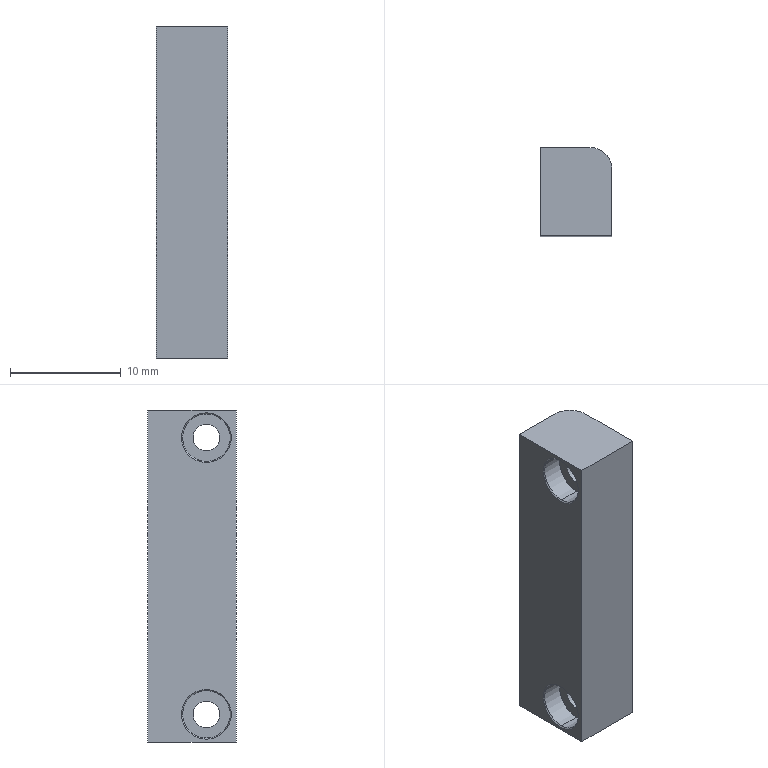Part | SolidWorks | features HoleWzd 2, Chamfer 1, Extrusion 1, Fillet 1 | 1 solid | 27 faces | box 6.5 x 8 x 30 mm | volume 1393 mm3 | cylinder 13 | plane 10 | cone 4 | commonest cylinder face diameters 2.4 x4 3 x4 4.3 x4 4 x1
STEP:
#1=CARTESIAN_POINT('',(-3.153,-1.3,0.35));
#2=VERTEX_POINT('',#1);
#3=CARTESIAN_POINT('',(-3.153,-1.3,4.65));
#4=VERTEX_POINT('',#3);
#5=CARTESIAN_POINT('',(-3.153,-1.3,2.5));
#6=DIRECTION('',(-1.,0.,0.));
#7=DIRECTION('',(0.,0.,-1.));
#8=AXIS2_PLACEMENT_3D('',#5,#6,#7);
#9=CIRCLE('',#8,2.15);
#10=EDGE_CURVE('',#2,#4,#9,.T.);
#11=ORIENTED_EDGE('',*,*,#10,.F.);
#12=CARTESIAN_POINT('',(-3.25,-1.3,0.25));
#13=VERTEX_POINT('',#12);
#14=CARTESIAN_POINT('',(-3.153,-1.3,0.35));
#15=DIRECTION('',(-0.6947,0.,-0.7193));
#16=VECTOR('',#15,1000.);
#17=LINE('',#14,#16);
#18=EDGE_CURVE('',#2,#13,#17,.T.);
#19=ORIENTED_EDGE('',*,*,#18,.T.);
#20=CARTESIAN_POINT('',(-3.25,-1.3,4.75));
#21=VERTEX_POINT('',#20);
#22=CARTESIAN_POINT('',(-3.25,-1.3,2.5));
#23=DIRECTION('',(1.,0.,0.));
#24=DIRECTION('',(0.,0.,-1.));
#25=AXIS2_PLACEMENT_3D('',#22,#23,#24);
#26=CIRCLE('',#25,2.25);
#27=EDGE_CURVE('',#21,#13,#26,.T.);
#28=ORIENTED_EDGE('',*,*,#27,.F.);
#29=CARTESIAN_POINT('',(-3.153,-1.3,4.65));
#30=DIRECTION('',(-0.6947,0.,0.7193));
#31=VECTOR('',#30,1000.);
#32=LINE('',#29,#31);
#33=EDGE_CURVE('',#4,#21,#32,.T.);
#34=ORIENTED_EDGE('',*,*,#33,.F.);
#35=EDGE_LOOP('',(#11,#19,#28,#34));
#36=FACE_OUTER_BOUND('',#35,.T.);
#37=CARTESIAN_POINT('',(-3.153,-1.3,2.5));
#38=DIRECTION('',(-1.,0.,0.));
#39=DIRECTION('',(0.,0.,1.));
#40=AXIS2_PLACEMENT_3D('',#37,#38,#39);
#41=CONICAL_SURFACE('',#40,2.15,0.8029);
#42=ADVANCED_FACE('',(#36),#41,.F.);
#43=CARTESIAN_POINT('',(-3.153,-1.3,25.35));
#44=VERTEX_POINT('',#43);
#45=CARTESIAN_POINT('',(-3.153,-1.3,29.65));
#46=VERTEX_POINT('',#45);
#47=CARTESIAN_POINT('',(-3.153,-1.3,27.5));
#48=DIRECTION('',(-1.,0.,0.));
#49=DIRECTION('',(0.,0.,-1.));
#50=AXIS2_PLACEMENT_3D('',#47,#48,#49);
#51=CIRCLE('',#50,2.15);
#52=EDGE_CURVE('',#44,#46,#51,.T.);
#53=ORIENTED_EDGE('',*,*,#52,.F.);
#54=CARTESIAN_POINT('',(-3.25,-1.3,25.25));
#55=VERTEX_POINT('',#54);
#56=CARTESIAN_POINT('',(-3.153,-1.3,25.35));
#57=DIRECTION('',(-0.6947,0.,-0.7193));
#58=VECTOR('',#57,1000.);
#59=LINE('',#56,#58);
#60=EDGE_CURVE('',#44,#55,#59,.T.);
#61=ORIENTED_EDGE('',*,*,#60,.T.);
#62=CARTESIAN_POINT('',(-3.25,-1.3,29.75));
#63=VERTEX_POINT('',#62);
#64=CARTESIAN_POINT('',(-3.25,-1.3,27.5));
#65=DIRECTION('',(1.,0.,0.));
#66=DIRECTION('',(0.,0.,-1.));
#67=AXIS2_PLACEMENT_3D('',#64,#65,#66);
#68=CIRCLE('',#67,2.25);
#69=EDGE_CURVE('',#63,#55,#68,.T.);
#70=ORIENTED_EDGE('',*,*,#69,.F.);
#71=CARTESIAN_POINT('',(-3.153,-1.3,29.65));
#72=DIRECTION('',(-0.6947,0.,0.7193));
#73=VECTOR('',#72,1000.);
#74=LINE('',#71,#73);
#75=EDGE_CURVE('',#46,#63,#74,.T.);
#76=ORIENTED_EDGE('',*,*,#75,.F.);
#77=EDGE_LOOP('',(#53,#61,#70,#76));
#78=FACE_OUTER_BOUND('',#77,.T.);
#79=CARTESIAN_POINT('',(-3.153,-1.3,27.5));
#80=DIRECTION('',(-1.,0.,0.));
#81=DIRECTION('',(0.,0.,1.));
#82=AXIS2_PLACEMENT_3D('',#79,#80,#81);
#83=CONICAL_SURFACE('',#82,2.15,0.8029);
#84=ADVANCED_FACE('',(#78),#83,.F.);
#85=CARTESIAN_POINT('',(-1.25,-1.3,25.35));
#86=VERTEX_POINT('',#85);
#87=CARTESIAN_POINT('',(-1.25,-1.3,29.65));
#88=VERTEX_POINT('',#87);
#89=CARTESIAN_POINT('',(-1.25,-1.3,27.5));
#90=DIRECTION('',(-1.,0.,0.));
#91=DIRECTION('',(0.,0.,1.));
#92=AXIS2_PLACEMENT_3D('',#89,#90,#91);
#93=CIRCLE('',#92,2.15);
#94=EDGE_CURVE('',#86,#88,#93,.T.);
#95=ORIENTED_EDGE('',*,*,#94,.F.);
#96=CARTESIAN_POINT('',(-3.25,-1.3,25.35));
#97=DIRECTION('',(-1.,0.,0.));
#98=VECTOR('',#97,1000.);
#99=LINE('',#96,#98);
#100=EDGE_CURVE('',#86,#44,#99,.T.);
#101=ORIENTED_EDGE('',*,*,#100,.T.);
#102=ORIENTED_EDGE('',*,*,#52,.T.);
#103=CARTESIAN_POINT('',(-3.25,-1.3,29.65));
#104=DIRECTION('',(-1.,0.,0.));
#105=VECTOR('',#104,1000.);
#106=LINE('',#103,#105);
#107=EDGE_CURVE('',#88,#46,#106,.T.);
#108=ORIENTED_EDGE('',*,*,#107,.F.);
#109=EDGE_LOOP('',(#95,#101,#102,#108));
#110=FACE_OUTER_BOUND('',#109,.T.);
#111=CARTESIAN_POINT('',(-3.25,-1.3,27.5));
#112=DIRECTION('',(-1.,0.,0.));
#113=DIRECTION('',(0.,0.,1.));
#114=AXIS2_PLACEMENT_3D('',#111,#112,#113);
#115=CYLINDRICAL_SURFACE('',#114,2.15);
#116=ADVANCED_FACE('',(#110),#115,.F.);
#117=CARTESIAN_POINT('',(3.25,-1.3,26.3));
#118=VERTEX_POINT('',#117);
#119=CARTESIAN_POINT('',(3.25,-1.3,28.7));
#120=VERTEX_POINT('',#119);
#121=CARTESIAN_POINT('',(3.25,-1.3,27.5));
#122=DIRECTION('',(-1.,0.,0.));
#123=DIRECTION('',(0.,0.,1.));
#124=AXIS2_PLACEMENT_3D('',#121,#122,#123);
#125=CIRCLE('',#124,1.2);
#126=EDGE_CURVE('',#118,#120,#125,.T.);
#127=ORIENTED_EDGE('',*,*,#126,.F.);
#128=CARTESIAN_POINT('',(-1.25,-1.3,26.3));
#129=VERTEX_POINT('',#128);
#130=CARTESIAN_POINT('',(-3.25,-1.3,26.3));
#131=DIRECTION('',(-1.,0.,0.));
#132=VECTOR('',#131,1000.);
#133=LINE('',#130,#132);
#134=EDGE_CURVE('',#118,#129,#133,.T.);
#135=ORIENTED_EDGE('',*,*,#134,.T.);
#136=CARTESIAN_POINT('',(-1.25,-1.3,28.7));
#137=VERTEX_POINT('',#136);
#138=CARTESIAN_POINT('',(-1.25,-1.3,27.5));
#139=DIRECTION('',(-1.,0.,0.));
#140=DIRECTION('',(0.,0.,1.));
#141=AXIS2_PLACEMENT_3D('',#138,#139,#140);
#142=CIRCLE('',#141,1.2);
#143=EDGE_CURVE('',#129,#137,#142,.T.);
#144=ORIENTED_EDGE('',*,*,#143,.T.);
#145=CARTESIAN_POINT('',(-3.25,-1.3,28.7));
#146=DIRECTION('',(-1.,0.,0.));
#147=VECTOR('',#146,1000.);
#148=LINE('',#145,#147);
#149=EDGE_CURVE('',#120,#137,#148,.T.);
#150=ORIENTED_EDGE('',*,*,#149,.F.);
#151=EDGE_LOOP('',(#127,#135,#144,#150));
#152=FACE_OUTER_BOUND('',#151,.T.);
#153=CARTESIAN_POINT('',(-3.25,-1.3,27.5));
#154=DIRECTION('',(-1.,0.,0.));
#155=DIRECTION('',(0.,0.,1.));
#156=AXIS2_PLACEMENT_3D('',#153,#154,#155);
#157=CYLINDRICAL_SURFACE('',#156,1.2);
#158=ADVANCED_FACE('',(#152),#157,.F.);
#159=CARTESIAN_POINT('',(-1.25,-1.3,0.35));
#160=VERTEX_POINT('',#159);
#161=CARTESIAN_POINT('',(-1.25,-1.3,4.65));
#162=VERTEX_POINT('',#161);
#163=CARTESIAN_POINT('',(-1.25,-1.3,2.5));
#164=DIRECTION('',(-1.,0.,0.));
#165=DIRECTION('',(0.,0.,1.));
#166=AXIS2_PLACEMENT_3D('',#163,#164,#165);
#167=CIRCLE('',#166,2.15);
#168=EDGE_CURVE('',#160,#162,#167,.T.);
#169=ORIENTED_EDGE('',*,*,#168,.F.);
#170=CARTESIAN_POINT('',(-3.25,-1.3,0.35));
#171=DIRECTION('',(-1.,0.,0.));
#172=VECTOR('',#171,1000.);
#173=LINE('',#170,#172);
#174=EDGE_CURVE('',#160,#2,#173,.T.);
#175=ORIENTED_EDGE('',*,*,#174,.T.);
#176=ORIENTED_EDGE('',*,*,#10,.T.);
#177=CARTESIAN_POINT('',(-3.25,-1.3,4.65));
#178=DIRECTION('',(-1.,0.,0.));
#179=VECTOR('',#178,1000.);
#180=LINE('',#177,#179);
#181=EDGE_CURVE('',#162,#4,#180,.T.);
#182=ORIENTED_EDGE('',*,*,#181,.F.);
#183=EDGE_LOOP('',(#169,#175,#176,#182));
#184=FACE_OUTER_BOUND('',#183,.T.);
#185=CARTESIAN_POINT('',(-3.25,-1.3,2.5));
#186=DIRECTION('',(-1.,0.,0.));
#187=DIRECTION('',(0.,0.,1.));
#188=AXIS2_PLACEMENT_3D('',#185,#186,#187);
#189=CYLINDRICAL_SURFACE('',#188,2.15);
#190=ADVANCED_FACE('',(#184),#189,.F.);
#191=CARTESIAN_POINT('',(3.25,-1.3,1.3));
#192=VERTEX_POINT('',#191);
#193=CARTESIAN_POINT('',(3.25,-1.3,3.7));
#194=VERTEX_POINT('',#193);
#195=CARTESIAN_POINT('',(3.25,-1.3,2.5));
#196=DIRECTION('',(-1.,0.,0.));
#197=DIRECTION('',(0.,0.,1.));
#198=AXIS2_PLACEMENT_3D('',#195,#196,#197);
#199=CIRCLE('',#198,1.2);
#200=EDGE_CURVE('',#192,#194,#199,.T.);
#201=ORIENTED_EDGE('',*,*,#200,.F.);
#202=CARTESIAN_POINT('',(-1.25,-1.3,1.3));
#203=VERTEX_POINT('',#202);
#204=CARTESIAN_POINT('',(-3.25,-1.3,1.3));
#205=DIRECTION('',(-1.,0.,0.));
#206=VECTOR('',#205,1000.);
#207=LINE('',#204,#206);
#208=EDGE_CURVE('',#192,#203,#207,.T.);
#209=ORIENTED_EDGE('',*,*,#208,.T.);
#210=CARTESIAN_POINT('',(-1.25,-1.3,3.7));
#211=VERTEX_POINT('',#210);
#212=CARTESIAN_POINT('',(-1.25,-1.3,2.5));
#213=DIRECTION('',(-1.,0.,0.));
#214=DIRECTION('',(0.,0.,1.));
#215=AXIS2_PLACEMENT_3D('',#212,#213,#214);
#216=CIRCLE('',#215,1.2);
#217=EDGE_CURVE('',#203,#211,#216,.T.);
#218=ORIENTED_EDGE('',*,*,#217,.T.);
#219=CARTESIAN_POINT('',(-3.25,-1.3,3.7));
#220=DIRECTION('',(-1.,0.,0.));
#221=VECTOR('',#220,1000.);
#222=LINE('',#219,#221);
#223=EDGE_CURVE('',#194,#211,#222,.T.);
#224=ORIENTED_EDGE('',*,*,#223,.F.);
#225=EDGE_LOOP('',(#201,#209,#218,#224));
#226=FACE_OUTER_BOUND('',#225,.T.);
#227=CARTESIAN_POINT('',(-3.25,-1.3,2.5));
#228=DIRECTION('',(-1.,0.,0.));
#229=DIRECTION('',(0.,0.,1.));
#230=AXIS2_PLACEMENT_3D('',#227,#228,#229);
#231=CYLINDRICAL_SURFACE('',#230,1.2);
#232=ADVANCED_FACE('',(#226),#231,.F.);
#233=CARTESIAN_POINT('',(0.25,-1.3,10.5));
#234=VERTEX_POINT('',#233);
#235=CARTESIAN_POINT('',(0.25,-1.3,7.5));
#236=VERTEX_POINT('',#235);
#237=CARTESIAN_POINT('',(0.25,-1.3,9.));
#238=DIRECTION('',(1.,0.,0.));
#239=DIRECTION('',(0.,0.,-1.));
#240=AXIS2_PLACEMENT_3D('',#237,#238,#239);
#241=CIRCLE('',#240,1.5);
#242=EDGE_CURVE('',#234,#236,#241,.T.);
#243=ORIENTED_EDGE('',*,*,#242,.F.);
#244=CARTESIAN_POINT('',(3.25,-1.3,10.5));
#245=VERTEX_POINT('',#244);
#246=CARTESIAN_POINT('',(3.25,-1.3,10.5));
#247=DIRECTION('',(1.,0.,0.));
#248=VECTOR('',#247,1000.);
#249=LINE('',#246,#248);
#250=EDGE_CURVE('',#234,#245,#249,.T.);
#251=ORIENTED_EDGE('',*,*,#250,.T.);
#252=CARTESIAN_POINT('',(3.25,-1.3,7.5));
#253=VERTEX_POINT('',#252);
#254=CARTESIAN_POINT('',(3.25,-1.3,9.));
#255=DIRECTION('',(1.,0.,0.));
#256=DIRECTION('',(0.,0.,-1.));
#257=AXIS2_PLACEMENT_3D('',#254,#255,#256);
#258=CIRCLE('',#257,1.5);
#259=EDGE_CURVE('',#245,#253,#258,.T.);
#260=ORIENTED_EDGE('',*,*,#259,.T.);
#261=CARTESIAN_POINT('',(3.25,-1.3,7.5));
#262=DIRECTION('',(1.,0.,0.));
#263=VECTOR('',#262,1000.);
#264=LINE('',#261,#263);
#265=EDGE_CURVE('',#236,#253,#264,.T.);
#266=ORIENTED_EDGE('',*,*,#265,.F.);
#267=EDGE_LOOP('',(#243,#251,#260,#266));
#268=FACE_OUTER_BOUND('',#267,.T.);
#269=CARTESIAN_POINT('',(3.25,-1.3,9.));
#270=DIRECTION('',(1.,0.,0.));
#271=DIRECTION('',(0.,0.,-1.));
#272=AXIS2_PLACEMENT_3D('',#269,#270,#271);
#273=CYLINDRICAL_SURFACE('',#272,1.5);
#274=ADVANCED_FACE('',(#268),#273,.F.);
#275=CARTESIAN_POINT('',(0.25,-1.3,22.5));
#276=VERTEX_POINT('',#275);
#277=CARTESIAN_POINT('',(0.25,-1.3,19.5));
#278=VERTEX_POINT('',#277);
#279=CARTESIAN_POINT('',(0.25,-1.3,21.));
#280=DIRECTION('',(1.,0.,0.));
#281=DIRECTION('',(0.,0.,-1.));
#282=AXIS2_PLACEMENT_3D('',#279,#280,#281);
#283=CIRCLE('',#282,1.5);
#284=EDGE_CURVE('',#276,#278,#283,.T.);
#285=ORIENTED_EDGE('',*,*,#284,.F.);
#286=CARTESIAN_POINT('',(3.25,-1.3,22.5));
#287=VERTEX_POINT('',#286);
#288=CARTESIAN_POINT('',(3.25,-1.3,22.5));
#289=DIRECTION('',(1.,0.,0.));
#290=VECTOR('',#289,1000.);
#291=LINE('',#288,#290);
#292=EDGE_CURVE('',#276,#287,#291,.T.);
#293=ORIENTED_EDGE('',*,*,#292,.T.);
#294=CARTESIAN_POINT('',(3.25,-1.3,19.5));
#295=VERTEX_POINT('',#294);
#296=CARTESIAN_POINT('',(3.25,-1.3,21.));
#297=DIRECTION('',(1.,0.,0.));
#298=DIRECTION('',(0.,0.,-1.));
#299=AXIS2_PLACEMENT_3D('',#296,#297,#298);
#300=CIRCLE('',#299,1.5);
#301=EDGE_CURVE('',#287,#295,#300,.T.);
#302=ORIENTED_EDGE('',*,*,#301,.T.);
#303=CARTESIAN_POINT('',(3.25,-1.3,19.5));
#304=DIRECTION('',(1.,0.,0.));
#305=VECTOR('',#304,1000.);
#306=LINE('',#303,#305);
#307=EDGE_CURVE('',#278,#295,#306,.T.);
#308=ORIENTED_EDGE('',*,*,#307,.F.);
#309=EDGE_LOOP('',(#285,#293,#302,#308));
#310=FACE_OUTER_BOUND('',#309,.T.);
#311=CARTESIAN_POINT('',(3.25,-1.3,21.));
#312=DIRECTION('',(1.,0.,0.));
#313=DIRECTION('',(0.,0.,-1.));
#314=AXIS2_PLACEMENT_3D('',#311,#312,#313);
#315=CYLINDRICAL_SURFACE('',#314,1.5);
#316=ADVANCED_FACE('',(#310),#315,.F.);
#317=CARTESIAN_POINT('',(3.25,-4.,30.));
#318=VERTEX_POINT('',#317);
#319=CARTESIAN_POINT('',(3.25,-4.,0.));
#320=VERTEX_POINT('',#319);
#321=CARTESIAN_POINT('',(3.25,-4.,30.));
#322=DIRECTION('',(0.,0.,-1.));
#323=VECTOR('',#322,1000.);
#324=LINE('',#321,#323);
#325=EDGE_CURVE('',#318,#320,#324,.T.);
#326=ORIENTED_EDGE('',*,*,#325,.F.);
#327=CARTESIAN_POINT('',(-3.25,-4.,30.));
#328=VERTEX_POINT('',#327);
#329=CARTESIAN_POINT('',(-3.25,-4.,30.));
#330=DIRECTION('',(1.,0.,0.));
#331=VECTOR('',#330,1000.);
#332=LINE('',#329,#331);
#333=EDGE_CURVE('',#328,#318,#332,.T.);
#334=ORIENTED_EDGE('',*,*,#333,.F.);
#335=CARTESIAN_POINT('',(-3.25,-4.,0.));
#336=VERTEX_POINT('',#335);
#337=CARTESIAN_POINT('',(-3.25,-4.,30.));
#338=DIRECTION('',(0.,0.,-1.));
#339=VECTOR('',#338,1000.);
#340=LINE('',#337,#339);
#341=EDGE_CURVE('',#328,#336,#340,.T.);
#342=ORIENTED_EDGE('',*,*,#341,.T.);
#343=CARTESIAN_POINT('',(-3.25,-4.,0.));
#344=DIRECTION('',(1.,0.,0.));
#345=VECTOR('',#344,1000.);
#346=LINE('',#343,#345);
#347=EDGE_CURVE('',#336,#320,#346,.T.);
#348=ORIENTED_EDGE('',*,*,#347,.T.);
#349=EDGE_LOOP('',(#326,#334,#342,#348));
#350=FACE_OUTER_BOUND('',#349,.T.);
#351=CARTESIAN_POINT('',(-3.25,-4.,30.));
#352=DIRECTION('',(0.,-1.,0.));
#353=DIRECTION('',(0.,0.,-1.));
#354=AXIS2_PLACEMENT_3D('',#351,#352,#353);
#355=PLANE('',#354);
#356=ADVANCED_FACE('',(#350),#355,.T.);
#357=CARTESIAN_POINT('',(3.25,2.,30.));
#358=VERTEX_POINT('',#357);
#359=CARTESIAN_POINT('',(3.25,4.,30.));
#360=DIRECTION('',(0.,-1.,0.));
#361=VECTOR('',#360,1000.);
#362=LINE('',#359,#361);
#363=EDGE_CURVE('',#358,#318,#362,.T.);
#364=ORIENTED_EDGE('',*,*,#363,.F.);
#365=CARTESIAN_POINT('',(1.25,4.,30.));
#366=VERTEX_POINT('',#365);
#367=CARTESIAN_POINT('',(1.25,2.,30.));
#368=DIRECTION('',(0.,0.,1.));
#369=DIRECTION('',(1.,0.,0.));
#370=AXIS2_PLACEMENT_3D('',#367,#368,#369);
#371=CIRCLE('',#370,2.);
#372=EDGE_CURVE('',#358,#366,#371,.T.);
#373=ORIENTED_EDGE('',*,*,#372,.T.);
#374=CARTESIAN_POINT('',(-3.25,4.,30.));
#375=VERTEX_POINT('',#374);
#376=CARTESIAN_POINT('',(-3.25,4.,30.));
#377=DIRECTION('',(1.,0.,0.));
#378=VECTOR('',#377,1000.);
#379=LINE('',#376,#378);
#380=EDGE_CURVE('',#375,#366,#379,.T.);
#381=ORIENTED_EDGE('',*,*,#380,.F.);
#382=CARTESIAN_POINT('',(-3.25,4.,30.));
#383=DIRECTION('',(0.,-1.,0.));
#384=VECTOR('',#383,1000.);
#385=LINE('',#382,#384);
#386=EDGE_CURVE('',#375,#328,#385,.T.);
#387=ORIENTED_EDGE('',*,*,#386,.T.);
#388=ORIENTED_EDGE('',*,*,#333,.T.);
#389=EDGE_LOOP('',(#364,#373,#381,#387,#388));
#390=FACE_OUTER_BOUND('',#389,.T.);
#391=CARTESIAN_POINT('',(-3.25,4.,30.));
#392=DIRECTION('',(0.,0.,1.));
#393=DIRECTION('',(1.,0.,0.));
#394=AXIS2_PLACEMENT_3D('',#391,#392,#393);
#395=PLANE('',#394);
#396=ADVANCED_FACE('',(#390),#395,.T.);
#397=ORIENTED_EDGE('',*,*,#380,.T.);
#398=CARTESIAN_POINT('',(1.25,4.,0.));
#399=VERTEX_POINT('',#398);
#400=CARTESIAN_POINT('',(1.25,4.,0.));
#401=DIRECTION('',(0.,0.,-1.));
#402=VECTOR('',#401,1000.);
#403=LINE('',#400,#402);
#404=EDGE_CURVE('',#366,#399,#403,.T.);
#405=ORIENTED_EDGE('',*,*,#404,.T.);
#406=CARTESIAN_POINT('',(-3.25,4.,0.));
#407=VERTEX_POINT('',#406);
#408=CARTESIAN_POINT('',(-3.25,4.,0.));
#409=DIRECTION('',(1.,0.,0.));
#410=VECTOR('',#409,1000.);
#411=LINE('',#408,#410);
#412=EDGE_CURVE('',#407,#399,#411,.T.);
#413=ORIENTED_EDGE('',*,*,#412,.F.);
#414=CARTESIAN_POINT('',(-3.25,4.,0.));
#415=DIRECTION('',(0.,0.,1.));
#416=VECTOR('',#415,1000.);
#417=LINE('',#414,#416);
#418=EDGE_CURVE('',#407,#375,#417,.T.);
#419=ORIENTED_EDGE('',*,*,#418,.T.);
#420=EDGE_LOOP('',(#397,#405,#413,#419));
#421=FACE_OUTER_BOUND('',#420,.T.);
#422=CARTESIAN_POINT('',(-3.25,4.,0.));
#423=DIRECTION('',(0.,1.,0.));
#424=DIRECTION('',(0.,0.,1.));
#425=AXIS2_PLACEMENT_3D('',#422,#423,#424);
#426=PLANE('',#425);
#427=ADVANCED_FACE('',(#421),#426,.T.);
#428=ORIENTED_EDGE('',*,*,#412,.T.);
#429=CARTESIAN_POINT('',(3.25,2.,0.));
#430=VERTEX_POINT('',#429);
#431=CARTESIAN_POINT('',(1.25,2.,0.));
#432=DIRECTION('',(0.,0.,-1.));
#433=DIRECTION('',(-1.,0.,0.));
#434=AXIS2_PLACEMENT_3D('',#431,#432,#433);
#435=CIRCLE('',#434,2.);
#436=EDGE_CURVE('',#399,#430,#435,.T.);
#437=ORIENTED_EDGE('',*,*,#436,.T.);
#438=CARTESIAN_POINT('',(3.25,-4.,0.));
#439=DIRECTION('',(0.,1.,0.));
#440=VECTOR('',#439,1000.);
#441=LINE('',#438,#440);
#442=EDGE_CURVE('',#320,#430,#441,.T.);
#443=ORIENTED_EDGE('',*,*,#442,.F.);
#444=ORIENTED_EDGE('',*,*,#347,.F.);
#445=CARTESIAN_POINT('',(-3.25,-4.,0.));
#446=DIRECTION('',(0.,1.,0.));
#447=VECTOR('',#446,1000.);
#448=LINE('',#445,#447);
#449=EDGE_CURVE('',#336,#407,#448,.T.);
#450=ORIENTED_EDGE('',*,*,#449,.T.);
#451=EDGE_LOOP('',(#428,#437,#443,#444,#450));
#452=FACE_OUTER_BOUND('',#451,.T.);
#453=CARTESIAN_POINT('',(-3.25,-4.,0.));
#454=DIRECTION('',(0.,0.,-1.));
#455=DIRECTION('',(-1.,0.,0.));
#456=AXIS2_PLACEMENT_3D('',#453,#454,#455);
#457=PLANE('',#456);
#458=ADVANCED_FACE('',(#452),#457,.T.);
#459=ORIENTED_EDGE('',*,*,#69,.T.);
#460=CARTESIAN_POINT('',(-3.25,-1.3,27.5));
#461=DIRECTION('',(1.,0.,0.));
#462=DIRECTION('',(0.,0.,-1.));
#463=AXIS2_PLACEMENT_3D('',#460,#461,#462);
#464=CIRCLE('',#463,2.25);
#465=EDGE_CURVE('',#55,#63,#464,.T.);
#466=ORIENTED_EDGE('',*,*,#465,.T.);
#467=EDGE_LOOP('',(#459,#466));
#468=FACE_BOUND('',#467,.T.);
#469=ORIENTED_EDGE('',*,*,#27,.T.);
#470=CARTESIAN_POINT('',(-3.25,-1.3,2.5));
#471=DIRECTION('',(1.,0.,0.));
#472=DIRECTION('',(0.,0.,-1.));
#473=AXIS2_PLACEMENT_3D('',#470,#471,#472);
#474=CIRCLE('',#473,2.25);
#475=EDGE_CURVE('',#13,#21,#474,.T.);
#476=ORIENTED_EDGE('',*,*,#475,.T.);
#477=EDGE_LOOP('',(#469,#476));
#478=FACE_BOUND('',#477,.T.);
#479=ORIENTED_EDGE('',*,*,#341,.F.);
#480=ORIENTED_EDGE('',*,*,#386,.F.);
#481=ORIENTED_EDGE('',*,*,#418,.F.);
#482=ORIENTED_EDGE('',*,*,#449,.F.);
#483=EDGE_LOOP('',(#479,#480,#481,#482));
#484=FACE_OUTER_BOUND('',#483,.T.);
#485=CARTESIAN_POINT('',(-3.25,0.,0.));
#486=DIRECTION('',(1.,0.,0.));
#487=DIRECTION('',(0.,0.,-1.));
#488=AXIS2_PLACEMENT_3D('',#485,#486,#487);
#489=PLANE('',#488);
#490=ADVANCED_FACE('',(#468,#478,#484),#489,.F.);
#491=CARTESIAN_POINT('',(3.25,-1.3,27.5));
#492=DIRECTION('',(-1.,0.,0.));
#493=DIRECTION('',(0.,0.,1.));
#494=AXIS2_PLACEMENT_3D('',#491,#492,#493);
#495=CIRCLE('',#494,1.2);
#496=EDGE_CURVE('',#120,#118,#495,.T.);
#497=ORIENTED_EDGE('',*,*,#496,.T.);
#498=ORIENTED_EDGE('',*,*,#126,.T.);
#499=EDGE_LOOP('',(#497,#498));
#500=FACE_BOUND('',#499,.T.);
#501=CARTESIAN_POINT('',(3.25,-1.3,2.5));
#502=DIRECTION('',(-1.,0.,0.));
#503=DIRECTION('',(0.,0.,1.));
#504=AXIS2_PLACEMENT_3D('',#501,#502,#503);
#505=CIRCLE('',#504,1.2);
#506=EDGE_CURVE('',#194,#192,#505,.T.);
#507=ORIENTED_EDGE('',*,*,#506,.T.);
#508=ORIENTED_EDGE('',*,*,#200,.T.);
#509=EDGE_LOOP('',(#507,#508));
#510=FACE_BOUND('',#509,.T.);
#511=CARTESIAN_POINT('',(3.25,-1.3,9.));
#512=DIRECTION('',(1.,0.,0.));
#513=DIRECTION('',(0.,0.,-1.));
#514=AXIS2_PLACEMENT_3D('',#511,#512,#513);
#515=CIRCLE('',#514,1.5);
#516=EDGE_CURVE('',#253,#245,#515,.T.);
#517=ORIENTED_EDGE('',*,*,#516,.F.);
#518=ORIENTED_EDGE('',*,*,#259,.F.);
#519=EDGE_LOOP('',(#517,#518));
#520=FACE_BOUND('',#519,.T.);
#521=CARTESIAN_POINT('',(3.25,-1.3,21.));
#522=DIRECTION('',(1.,0.,0.));
#523=DIRECTION('',(0.,0.,-1.));
#524=AXIS2_PLACEMENT_3D('',#521,#522,#523);
#525=CIRCLE('',#524,1.5);
#526=EDGE_CURVE('',#295,#287,#525,.T.);
#527=ORIENTED_EDGE('',*,*,#526,.F.);
#528=ORIENTED_EDGE('',*,*,#301,.F.);
#529=EDGE_LOOP('',(#527,#528));
#530=FACE_BOUND('',#529,.T.);
#531=ORIENTED_EDGE('',*,*,#442,.T.);
#532=CARTESIAN_POINT('',(3.25,2.,0.));
#533=DIRECTION('',(0.,0.,1.));
#534=VECTOR('',#533,1000.);
#535=LINE('',#532,#534);
#536=EDGE_CURVE('',#430,#358,#535,.T.);
#537=ORIENTED_EDGE('',*,*,#536,.T.);
#538=ORIENTED_EDGE('',*,*,#363,.T.);
#539=ORIENTED_EDGE('',*,*,#325,.T.);
#540=EDGE_LOOP('',(#531,#537,#538,#539));
#541=FACE_OUTER_BOUND('',#540,.T.);
#542=CARTESIAN_POINT('',(3.25,0.,0.));
#543=DIRECTION('',(1.,0.,0.));
#544=DIRECTION('',(0.,0.,-1.));
#545=AXIS2_PLACEMENT_3D('',#542,#543,#544);
#546=PLANE('',#545);
#547=ADVANCED_FACE('',(#500,#510,#520,#530,#541),#546,.T.);
#548=CARTESIAN_POINT('',(0.25,-1.3,21.));
#549=DIRECTION('',(1.,0.,0.));
#550=DIRECTION('',(0.,0.,-1.));
#551=AXIS2_PLACEMENT_3D('',#548,#549,#550);
#552=CIRCLE('',#551,1.5);
#553=EDGE_CURVE('',#278,#276,#552,.T.);
#554=ORIENTED_EDGE('',*,*,#553,.T.);
#555=ORIENTED_EDGE('',*,*,#284,.T.);
#556=EDGE_LOOP('',(#554,#555));
#557=FACE_OUTER_BOUND('',#556,.T.);
#558=CARTESIAN_POINT('',(0.25,-1.3,21.));
#559=DIRECTION('',(-1.,0.,0.));
#560=DIRECTION('',(0.,0.,1.));
#561=AXIS2_PLACEMENT_3D('',#558,#559,#560);
#562=PLANE('',#561);
#563=ADVANCED_FACE('',(#557),#562,.F.);
#564=ORIENTED_EDGE('',*,*,#292,.F.);
#565=ORIENTED_EDGE('',*,*,#553,.F.);
#566=ORIENTED_EDGE('',*,*,#307,.T.);
#567=ORIENTED_EDGE('',*,*,#526,.T.);
#568=EDGE_LOOP('',(#564,#565,#566,#567));
#569=FACE_OUTER_BOUND('',#568,.T.);
#570=CARTESIAN_POINT('',(3.25,-1.3,21.));
#571=DIRECTION('',(1.,0.,0.));
#572=DIRECTION('',(0.,0.,-1.));
#573=AXIS2_PLACEMENT_3D('',#570,#571,#572);
#574=CYLINDRICAL_SURFACE('',#573,1.5);
#575=ADVANCED_FACE('',(#569),#574,.F.);
#576=CARTESIAN_POINT('',(0.25,-1.3,9.));
#577=DIRECTION('',(1.,0.,0.));
#578=DIRECTION('',(0.,0.,-1.));
#579=AXIS2_PLACEMENT_3D('',#576,#577,#578);
#580=CIRCLE('',#579,1.5);
#581=EDGE_CURVE('',#236,#234,#580,.T.);
#582=ORIENTED_EDGE('',*,*,#581,.T.);
#583=ORIENTED_EDGE('',*,*,#242,.T.);
#584=EDGE_LOOP('',(#582,#583));
#585=FACE_OUTER_BOUND('',#584,.T.);
#586=CARTESIAN_POINT('',(0.25,-1.3,9.));
#587=DIRECTION('',(-1.,0.,0.));
#588=DIRECTION('',(0.,0.,1.));
#589=AXIS2_PLACEMENT_3D('',#586,#587,#588);
#590=PLANE('',#589);
#591=ADVANCED_FACE('',(#585),#590,.F.);
#592=ORIENTED_EDGE('',*,*,#250,.F.);
#593=ORIENTED_EDGE('',*,*,#581,.F.);
#594=ORIENTED_EDGE('',*,*,#265,.T.);
#595=ORIENTED_EDGE('',*,*,#516,.T.);
#596=EDGE_LOOP('',(#592,#593,#594,#595));
#597=FACE_OUTER_BOUND('',#596,.T.);
#598=CARTESIAN_POINT('',(3.25,-1.3,9.));
#599=DIRECTION('',(1.,0.,0.));
#600=DIRECTION('',(0.,0.,-1.));
#601=AXIS2_PLACEMENT_3D('',#598,#599,#600);
#602=CYLINDRICAL_SURFACE('',#601,1.5);
#603=ADVANCED_FACE('',(#597),#602,.F.);
#604=ORIENTED_EDGE('',*,*,#208,.F.);
#605=ORIENTED_EDGE('',*,*,#506,.F.);
#606=ORIENTED_EDGE('',*,*,#223,.T.);
#607=CARTESIAN_POINT('',(-1.25,-1.3,2.5));
#608=DIRECTION('',(-1.,0.,0.));
#609=DIRECTION('',(0.,0.,1.));
#610=AXIS2_PLACEMENT_3D('',#607,#608,#609);
#611=CIRCLE('',#610,1.2);
#612=EDGE_CURVE('',#211,#203,#611,.T.);
#613=ORIENTED_EDGE('',*,*,#612,.T.);
#614=EDGE_LOOP('',(#604,#605,#606,#613));
#615=FACE_OUTER_BOUND('',#614,.T.);
#616=CARTESIAN_POINT('',(-3.25,-1.3,2.5));
#617=DIRECTION('',(-1.,0.,0.));
#618=DIRECTION('',(0.,0.,1.));
#619=AXIS2_PLACEMENT_3D('',#616,#617,#618);
#620=CYLINDRICAL_SURFACE('',#619,1.2);
#621=ADVANCED_FACE('',(#615),#620,.F.);
#622=ORIENTED_EDGE('',*,*,#612,.F.);
#623=ORIENTED_EDGE('',*,*,#217,.F.);
#624=EDGE_LOOP('',(#622,#623));
#625=FACE_BOUND('',#624,.T.);
#626=CARTESIAN_POINT('',(-1.25,-1.3,2.5));
#627=DIRECTION('',(-1.,0.,0.));
#628=DIRECTION('',(0.,0.,1.));
#629=AXIS2_PLACEMENT_3D('',#626,#627,#628);
#630=CIRCLE('',#629,2.15);
#631=EDGE_CURVE('',#162,#160,#630,.T.);
#632=ORIENTED_EDGE('',*,*,#631,.T.);
#633=ORIENTED_EDGE('',*,*,#168,.T.);
#634=EDGE_LOOP('',(#632,#633));
#635=FACE_OUTER_BOUND('',#634,.T.);
#636=CARTESIAN_POINT('',(-1.25,-0.1,2.5));
#637=DIRECTION('',(1.,0.,0.));
#638=DIRECTION('',(0.,0.,-1.));
#639=AXIS2_PLACEMENT_3D('',#636,#637,#638);
#640=PLANE('',#639);
#641=ADVANCED_FACE('',(#625,#635),#640,.F.);
#642=ORIENTED_EDGE('',*,*,#174,.F.);
#643=ORIENTED_EDGE('',*,*,#631,.F.);
#644=ORIENTED_EDGE('',*,*,#181,.T.);
#645=CARTESIAN_POINT('',(-3.153,-1.3,2.5));
#646=DIRECTION('',(-1.,0.,0.));
#647=DIRECTION('',(0.,0.,-1.));
#648=AXIS2_PLACEMENT_3D('',#645,#646,#647);
#649=CIRCLE('',#648,2.15);
#650=EDGE_CURVE('',#4,#2,#649,.T.);
#651=ORIENTED_EDGE('',*,*,#650,.T.);
#652=EDGE_LOOP('',(#642,#643,#644,#651));
#653=FACE_OUTER_BOUND('',#652,.T.);
#654=CARTESIAN_POINT('',(-3.25,-1.3,2.5));
#655=DIRECTION('',(-1.,0.,0.));
#656=DIRECTION('',(0.,0.,1.));
#657=AXIS2_PLACEMENT_3D('',#654,#655,#656);
#658=CYLINDRICAL_SURFACE('',#657,2.15);
#659=ADVANCED_FACE('',(#653),#658,.F.);
#660=ORIENTED_EDGE('',*,*,#134,.F.);
#661=ORIENTED_EDGE('',*,*,#496,.F.);
#662=ORIENTED_EDGE('',*,*,#149,.T.);
#663=CARTESIAN_POINT('',(-1.25,-1.3,27.5));
#664=DIRECTION('',(-1.,0.,0.));
#665=DIRECTION('',(0.,0.,1.));
#666=AXIS2_PLACEMENT_3D('',#663,#664,#665);
#667=CIRCLE('',#666,1.2);
#668=EDGE_CURVE('',#137,#129,#667,.T.);
#669=ORIENTED_EDGE('',*,*,#668,.T.);
#670=EDGE_LOOP('',(#660,#661,#662,#669));
#671=FACE_OUTER_BOUND('',#670,.T.);
#672=CARTESIAN_POINT('',(-3.25,-1.3,27.5));
#673=DIRECTION('',(-1.,0.,0.));
#674=DIRECTION('',(0.,0.,1.));
#675=AXIS2_PLACEMENT_3D('',#672,#673,#674);
#676=CYLINDRICAL_SURFACE('',#675,1.2);
#677=ADVANCED_FACE('',(#671),#676,.F.);
#678=ORIENTED_EDGE('',*,*,#668,.F.);
#679=ORIENTED_EDGE('',*,*,#143,.F.);
#680=EDGE_LOOP('',(#678,#679));
#681=FACE_BOUND('',#680,.T.);
#682=CARTESIAN_POINT('',(-1.25,-1.3,27.5));
#683=DIRECTION('',(-1.,0.,0.));
#684=DIRECTION('',(0.,0.,1.));
#685=AXIS2_PLACEMENT_3D('',#682,#683,#684);
#686=CIRCLE('',#685,2.15);
#687=EDGE_CURVE('',#88,#86,#686,.T.);
#688=ORIENTED_EDGE('',*,*,#687,.T.);
#689=ORIENTED_EDGE('',*,*,#94,.T.);
#690=EDGE_LOOP('',(#688,#689));
#691=FACE_OUTER_BOUND('',#690,.T.);
#692=CARTESIAN_POINT('',(-1.25,-0.1,27.5));
#693=DIRECTION('',(1.,0.,0.));
#694=DIRECTION('',(0.,0.,-1.));
#695=AXIS2_PLACEMENT_3D('',#692,#693,#694);
#696=PLANE('',#695);
#697=ADVANCED_FACE('',(#681,#691),#696,.F.);
#698=ORIENTED_EDGE('',*,*,#100,.F.);
#699=ORIENTED_EDGE('',*,*,#687,.F.);
#700=ORIENTED_EDGE('',*,*,#107,.T.);
#701=CARTESIAN_POINT('',(-3.153,-1.3,27.5));
#702=DIRECTION('',(-1.,0.,0.));
#703=DIRECTION('',(0.,0.,-1.));
#704=AXIS2_PLACEMENT_3D('',#701,#702,#703);
#705=CIRCLE('',#704,2.15);
#706=EDGE_CURVE('',#46,#44,#705,.T.);
#707=ORIENTED_EDGE('',*,*,#706,.T.);
#708=EDGE_LOOP('',(#698,#699,#700,#707));
#709=FACE_OUTER_BOUND('',#708,.T.);
#710=CARTESIAN_POINT('',(-3.25,-1.3,27.5));
#711=DIRECTION('',(-1.,0.,0.));
#712=DIRECTION('',(0.,0.,1.));
#713=AXIS2_PLACEMENT_3D('',#710,#711,#712);
#714=CYLINDRICAL_SURFACE('',#713,2.15);
#715=ADVANCED_FACE('',(#709),#714,.F.);
#716=ORIENTED_EDGE('',*,*,#60,.F.);
#717=ORIENTED_EDGE('',*,*,#706,.F.);
#718=ORIENTED_EDGE('',*,*,#75,.T.);
#719=ORIENTED_EDGE('',*,*,#465,.F.);
#720=EDGE_LOOP('',(#716,#717,#718,#719));
#721=FACE_OUTER_BOUND('',#720,.T.);
#722=CARTESIAN_POINT('',(-3.153,-1.3,27.5));
#723=DIRECTION('',(-1.,0.,0.));
#724=DIRECTION('',(0.,0.,1.));
#725=AXIS2_PLACEMENT_3D('',#722,#723,#724);
#726=CONICAL_SURFACE('',#725,2.15,0.8029);
#727=ADVANCED_FACE('',(#721),#726,.F.);
#728=ORIENTED_EDGE('',*,*,#18,.F.);
#729=ORIENTED_EDGE('',*,*,#650,.F.);
#730=ORIENTED_EDGE('',*,*,#33,.T.);
#731=ORIENTED_EDGE('',*,*,#475,.F.);
#732=EDGE_LOOP('',(#728,#729,#730,#731));
#733=FACE_OUTER_BOUND('',#732,.T.);
#734=CARTESIAN_POINT('',(-3.153,-1.3,2.5));
#735=DIRECTION('',(-1.,0.,0.));
#736=DIRECTION('',(0.,0.,1.));
#737=AXIS2_PLACEMENT_3D('',#734,#735,#736);
#738=CONICAL_SURFACE('',#737,2.15,0.8029);
#739=ADVANCED_FACE('',(#733),#738,.F.);
#740=ORIENTED_EDGE('',*,*,#436,.F.);
#741=ORIENTED_EDGE('',*,*,#404,.F.);
#742=ORIENTED_EDGE('',*,*,#372,.F.);
#743=ORIENTED_EDGE('',*,*,#536,.F.);
#744=EDGE_LOOP('',(#740,#741,#742,#743));
#745=FACE_OUTER_BOUND('',#744,.T.);
#746=CARTESIAN_POINT('',(1.25,2.,0.));
#747=DIRECTION('',(0.,0.,1.));
#748=DIRECTION('',(1.,0.,0.));
#749=AXIS2_PLACEMENT_3D('',#746,#747,#748);
#750=CYLINDRICAL_SURFACE('',#749,2.);
#751=ADVANCED_FACE('',(#745),#750,.T.);
#752=CLOSED_SHELL('',(#42,#84,#116,#158,#190,#232,#274,#316,#356,#396,#427,#458,#490,#547,#563,#575,#591,#603,#621,#641,#659,#677,#697,#715,#727,#739,#751));
#753=MANIFOLD_SOLID_BREP('',#752);
#754=CARTESIAN_POINT('',(0.,0.,0.));
#755=DIRECTION('',(0.,0.,1.));
#756=DIRECTION('',(1.,0.,0.));
#757=AXIS2_PLACEMENT_3D('',#754,#755,#756);
#758=(LENGTH_UNIT()NAMED_UNIT(*)SI_UNIT(.MILLI.,.METRE.));
#759=UNCERTAINTY_MEASURE_WITH_UNIT(LENGTH_MEASURE(0.00001),#758,'','');
#760=(NAMED_UNIT(*)PLANE_ANGLE_UNIT()SI_UNIT($,.RADIAN.));
#761=(NAMED_UNIT(*)SI_UNIT($,.STERADIAN.)SOLID_ANGLE_UNIT());
#762=(GEOMETRIC_REPRESENTATION_CONTEXT(3)GLOBAL_UNCERTAINTY_ASSIGNED_CONTEXT((#759))GLOBAL_UNIT_ASSIGNED_CONTEXT((#758,#760,#761))REPRESENTATION_CONTEXT('',''));
#763=ADVANCED_BREP_SHAPE_REPRESENTATION('',(#753,#757),#762);